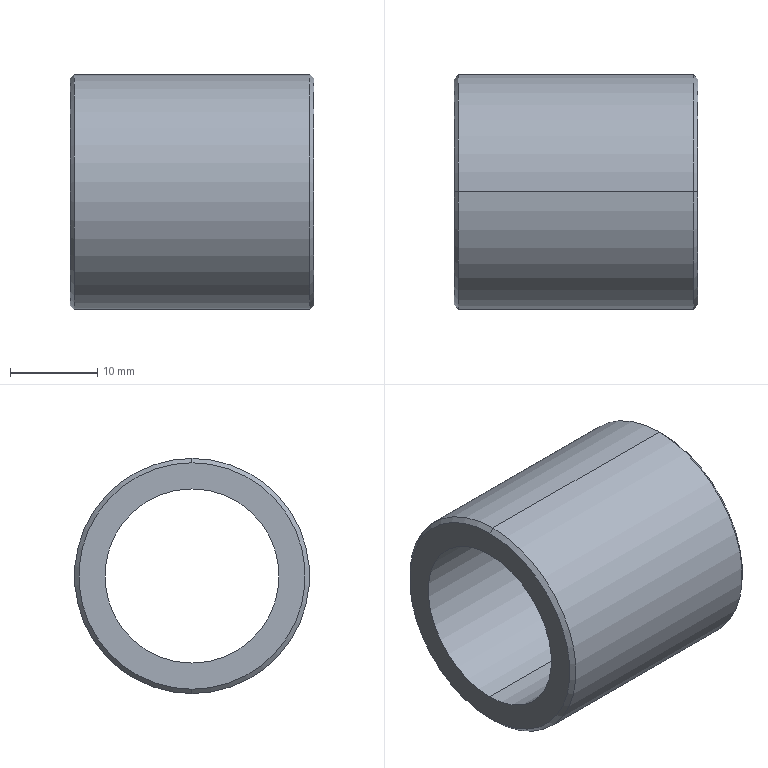Part | STEP file | CLBUS20-27-28.0-1 | 1 solid | 10 faces | box 28 x 27 x 27 mm | volume 7214 mm3 | cone 4 | cylinder 4 | plane 2 | commonest cylinder face diameters 20 x2 27 x2
STEP:
#1=CARTESIAN_POINT('',(28.,0.,-13.));
#2=VERTEX_POINT('',#1);
#3=CARTESIAN_POINT('',(28.,0.,13.));
#4=VERTEX_POINT('',#3);
#5=CARTESIAN_POINT('',(28.,0.,0.));
#6=DIRECTION('',(1.,0.,0.));
#7=DIRECTION('',(0.,0.,1.));
#8=AXIS2_PLACEMENT_3D('',#5,#6,#7);
#9=CIRCLE('',#8,13.);
#10=EDGE_CURVE('',#2,#4,#9,.T.);
#11=ORIENTED_EDGE('',*,*,#10,.F.);
#12=CARTESIAN_POINT('',(27.5,0.,-13.5));
#13=VERTEX_POINT('',#12);
#14=CARTESIAN_POINT('',(27.5,0.,-13.5));
#15=DIRECTION('',(-0.7071,0.,-0.7071));
#16=VECTOR('',#15,1000.);
#17=LINE('',#14,#16);
#18=EDGE_CURVE('',#2,#13,#17,.T.);
#19=ORIENTED_EDGE('',*,*,#18,.T.);
#20=CARTESIAN_POINT('',(27.5,0.,13.5));
#21=VERTEX_POINT('',#20);
#22=CARTESIAN_POINT('',(27.5,0.,0.));
#23=DIRECTION('',(-1.,0.,0.));
#24=DIRECTION('',(0.,0.,1.));
#25=AXIS2_PLACEMENT_3D('',#22,#23,#24);
#26=CIRCLE('',#25,13.5);
#27=EDGE_CURVE('',#21,#13,#26,.T.);
#28=ORIENTED_EDGE('',*,*,#27,.F.);
#29=CARTESIAN_POINT('',(27.5,0.,13.5));
#30=DIRECTION('',(-0.7071,0.,0.7071));
#31=VECTOR('',#30,1000.);
#32=LINE('',#29,#31);
#33=EDGE_CURVE('',#4,#21,#32,.T.);
#34=ORIENTED_EDGE('',*,*,#33,.F.);
#35=EDGE_LOOP('',(#11,#19,#28,#34));
#36=FACE_OUTER_BOUND('',#35,.T.);
#37=CARTESIAN_POINT('',(27.5,0.,0.));
#38=DIRECTION('',(-1.,0.,0.));
#39=DIRECTION('',(0.,0.,1.));
#40=AXIS2_PLACEMENT_3D('',#37,#38,#39);
#41=CONICAL_SURFACE('',#40,13.5,0.7854);
#42=ADVANCED_FACE('',(#36),#41,.T.);
#43=CARTESIAN_POINT('',(0.,0.,13.));
#44=VERTEX_POINT('',#43);
#45=CARTESIAN_POINT('',(0.,0.,-13.));
#46=VERTEX_POINT('',#45);
#47=CARTESIAN_POINT('',(0.,0.,0.));
#48=DIRECTION('',(-1.,0.,0.));
#49=DIRECTION('',(0.,0.,-1.));
#50=AXIS2_PLACEMENT_3D('',#47,#48,#49);
#51=CIRCLE('',#50,13.);
#52=EDGE_CURVE('',#44,#46,#51,.T.);
#53=ORIENTED_EDGE('',*,*,#52,.F.);
#54=CARTESIAN_POINT('',(0.5,0.,13.5));
#55=VERTEX_POINT('',#54);
#56=CARTESIAN_POINT('',(0.,0.,13.));
#57=DIRECTION('',(0.7071,0.,0.7071));
#58=VECTOR('',#57,1000.);
#59=LINE('',#56,#58);
#60=EDGE_CURVE('',#44,#55,#59,.T.);
#61=ORIENTED_EDGE('',*,*,#60,.T.);
#62=CARTESIAN_POINT('',(0.5,0.,-13.5));
#63=VERTEX_POINT('',#62);
#64=CARTESIAN_POINT('',(0.5,0.,0.));
#65=DIRECTION('',(1.,0.,0.));
#66=DIRECTION('',(0.,0.,-1.));
#67=AXIS2_PLACEMENT_3D('',#64,#65,#66);
#68=CIRCLE('',#67,13.5);
#69=EDGE_CURVE('',#63,#55,#68,.T.);
#70=ORIENTED_EDGE('',*,*,#69,.F.);
#71=CARTESIAN_POINT('',(0.,0.,-13.));
#72=DIRECTION('',(0.7071,0.,-0.7071));
#73=VECTOR('',#72,1000.);
#74=LINE('',#71,#73);
#75=EDGE_CURVE('',#46,#63,#74,.T.);
#76=ORIENTED_EDGE('',*,*,#75,.F.);
#77=EDGE_LOOP('',(#53,#61,#70,#76));
#78=FACE_OUTER_BOUND('',#77,.T.);
#79=CARTESIAN_POINT('',(0.,0.,0.));
#80=DIRECTION('',(1.,0.,0.));
#81=DIRECTION('',(0.,0.,-1.));
#82=AXIS2_PLACEMENT_3D('',#79,#80,#81);
#83=CONICAL_SURFACE('',#82,13.,0.7854);
#84=ADVANCED_FACE('',(#78),#83,.T.);
#85=ORIENTED_EDGE('',*,*,#27,.T.);
#86=CARTESIAN_POINT('',(0.,0.,-13.5));
#87=DIRECTION('',(-1.,0.,0.));
#88=VECTOR('',#87,1000.);
#89=LINE('',#86,#88);
#90=EDGE_CURVE('',#13,#63,#89,.T.);
#91=ORIENTED_EDGE('',*,*,#90,.T.);
#92=ORIENTED_EDGE('',*,*,#69,.T.);
#93=CARTESIAN_POINT('',(0.,0.,13.5));
#94=DIRECTION('',(-1.,0.,0.));
#95=VECTOR('',#94,1000.);
#96=LINE('',#93,#95);
#97=EDGE_CURVE('',#21,#55,#96,.T.);
#98=ORIENTED_EDGE('',*,*,#97,.F.);
#99=EDGE_LOOP('',(#85,#91,#92,#98));
#100=FACE_OUTER_BOUND('',#99,.T.);
#101=CARTESIAN_POINT('',(0.,0.,0.));
#102=DIRECTION('',(-1.,0.,0.));
#103=DIRECTION('',(0.,0.,1.));
#104=AXIS2_PLACEMENT_3D('',#101,#102,#103);
#105=CYLINDRICAL_SURFACE('',#104,13.5);
#106=ADVANCED_FACE('',(#100),#105,.T.);
#107=CARTESIAN_POINT('',(28.,0.,-10.));
#108=VERTEX_POINT('',#107);
#109=CARTESIAN_POINT('',(28.,0.,10.));
#110=VERTEX_POINT('',#109);
#111=CARTESIAN_POINT('',(28.,0.,0.));
#112=DIRECTION('',(-1.,0.,0.));
#113=DIRECTION('',(0.,0.,1.));
#114=AXIS2_PLACEMENT_3D('',#111,#112,#113);
#115=CIRCLE('',#114,10.);
#116=EDGE_CURVE('',#108,#110,#115,.T.);
#117=ORIENTED_EDGE('',*,*,#116,.F.);
#118=CARTESIAN_POINT('',(0.,0.,-10.));
#119=VERTEX_POINT('',#118);
#120=CARTESIAN_POINT('',(0.,0.,-10.));
#121=DIRECTION('',(-1.,0.,0.));
#122=VECTOR('',#121,1000.);
#123=LINE('',#120,#122);
#124=EDGE_CURVE('',#108,#119,#123,.T.);
#125=ORIENTED_EDGE('',*,*,#124,.T.);
#126=CARTESIAN_POINT('',(0.,0.,10.));
#127=VERTEX_POINT('',#126);
#128=CARTESIAN_POINT('',(0.,0.,0.));
#129=DIRECTION('',(-1.,0.,0.));
#130=DIRECTION('',(0.,0.,1.));
#131=AXIS2_PLACEMENT_3D('',#128,#129,#130);
#132=CIRCLE('',#131,10.);
#133=EDGE_CURVE('',#119,#127,#132,.T.);
#134=ORIENTED_EDGE('',*,*,#133,.T.);
#135=CARTESIAN_POINT('',(0.,0.,10.));
#136=DIRECTION('',(-1.,0.,0.));
#137=VECTOR('',#136,1000.);
#138=LINE('',#135,#137);
#139=EDGE_CURVE('',#110,#127,#138,.T.);
#140=ORIENTED_EDGE('',*,*,#139,.F.);
#141=EDGE_LOOP('',(#117,#125,#134,#140));
#142=FACE_OUTER_BOUND('',#141,.T.);
#143=CARTESIAN_POINT('',(0.,0.,0.));
#144=DIRECTION('',(-1.,0.,0.));
#145=DIRECTION('',(0.,0.,1.));
#146=AXIS2_PLACEMENT_3D('',#143,#144,#145);
#147=CYLINDRICAL_SURFACE('',#146,10.);
#148=ADVANCED_FACE('',(#142),#147,.F.);
#149=CARTESIAN_POINT('',(28.,0.,0.));
#150=DIRECTION('',(1.,0.,0.));
#151=DIRECTION('',(0.,0.,1.));
#152=AXIS2_PLACEMENT_3D('',#149,#150,#151);
#153=CIRCLE('',#152,13.);
#154=EDGE_CURVE('',#4,#2,#153,.T.);
#155=ORIENTED_EDGE('',*,*,#154,.T.);
#156=ORIENTED_EDGE('',*,*,#10,.T.);
#157=EDGE_LOOP('',(#155,#156));
#158=FACE_OUTER_BOUND('',#157,.T.);
#159=CARTESIAN_POINT('',(28.,0.,0.));
#160=DIRECTION('',(-1.,0.,0.));
#161=DIRECTION('',(0.,0.,1.));
#162=AXIS2_PLACEMENT_3D('',#159,#160,#161);
#163=CIRCLE('',#162,10.);
#164=EDGE_CURVE('',#110,#108,#163,.T.);
#165=ORIENTED_EDGE('',*,*,#164,.T.);
#166=ORIENTED_EDGE('',*,*,#116,.T.);
#167=EDGE_LOOP('',(#165,#166));
#168=FACE_BOUND('',#167,.T.);
#169=CARTESIAN_POINT('',(28.,13.5,0.));
#170=DIRECTION('',(-1.,0.,0.));
#171=DIRECTION('',(0.,0.,1.));
#172=AXIS2_PLACEMENT_3D('',#169,#170,#171);
#173=PLANE('',#172);
#174=ADVANCED_FACE('',(#158,#168),#173,.F.);
#175=ORIENTED_EDGE('',*,*,#124,.F.);
#176=ORIENTED_EDGE('',*,*,#164,.F.);
#177=ORIENTED_EDGE('',*,*,#139,.T.);
#178=CARTESIAN_POINT('',(0.,0.,0.));
#179=DIRECTION('',(-1.,0.,0.));
#180=DIRECTION('',(0.,0.,1.));
#181=AXIS2_PLACEMENT_3D('',#178,#179,#180);
#182=CIRCLE('',#181,10.);
#183=EDGE_CURVE('',#127,#119,#182,.T.);
#184=ORIENTED_EDGE('',*,*,#183,.T.);
#185=EDGE_LOOP('',(#175,#176,#177,#184));
#186=FACE_OUTER_BOUND('',#185,.T.);
#187=CARTESIAN_POINT('',(0.,0.,0.));
#188=DIRECTION('',(-1.,0.,0.));
#189=DIRECTION('',(0.,0.,1.));
#190=AXIS2_PLACEMENT_3D('',#187,#188,#189);
#191=CYLINDRICAL_SURFACE('',#190,10.);
#192=ADVANCED_FACE('',(#186),#191,.F.);
#193=CARTESIAN_POINT('',(0.,0.,0.));
#194=DIRECTION('',(-1.,0.,0.));
#195=DIRECTION('',(0.,0.,-1.));
#196=AXIS2_PLACEMENT_3D('',#193,#194,#195);
#197=CIRCLE('',#196,13.);
#198=EDGE_CURVE('',#46,#44,#197,.T.);
#199=ORIENTED_EDGE('',*,*,#198,.T.);
#200=ORIENTED_EDGE('',*,*,#52,.T.);
#201=EDGE_LOOP('',(#199,#200));
#202=FACE_OUTER_BOUND('',#201,.T.);
#203=ORIENTED_EDGE('',*,*,#183,.F.);
#204=ORIENTED_EDGE('',*,*,#133,.F.);
#205=EDGE_LOOP('',(#203,#204));
#206=FACE_BOUND('',#205,.T.);
#207=CARTESIAN_POINT('',(0.,10.,0.));
#208=DIRECTION('',(1.,0.,0.));
#209=DIRECTION('',(0.,0.,-1.));
#210=AXIS2_PLACEMENT_3D('',#207,#208,#209);
#211=PLANE('',#210);
#212=ADVANCED_FACE('',(#202,#206),#211,.F.);
#213=ORIENTED_EDGE('',*,*,#90,.F.);
#214=CARTESIAN_POINT('',(27.5,0.,0.));
#215=DIRECTION('',(-1.,0.,0.));
#216=DIRECTION('',(0.,0.,1.));
#217=AXIS2_PLACEMENT_3D('',#214,#215,#216);
#218=CIRCLE('',#217,13.5);
#219=EDGE_CURVE('',#13,#21,#218,.T.);
#220=ORIENTED_EDGE('',*,*,#219,.T.);
#221=ORIENTED_EDGE('',*,*,#97,.T.);
#222=CARTESIAN_POINT('',(0.5,0.,0.));
#223=DIRECTION('',(1.,0.,0.));
#224=DIRECTION('',(0.,0.,-1.));
#225=AXIS2_PLACEMENT_3D('',#222,#223,#224);
#226=CIRCLE('',#225,13.5);
#227=EDGE_CURVE('',#55,#63,#226,.T.);
#228=ORIENTED_EDGE('',*,*,#227,.T.);
#229=EDGE_LOOP('',(#213,#220,#221,#228));
#230=FACE_OUTER_BOUND('',#229,.T.);
#231=CARTESIAN_POINT('',(0.,0.,0.));
#232=DIRECTION('',(-1.,0.,0.));
#233=DIRECTION('',(0.,0.,1.));
#234=AXIS2_PLACEMENT_3D('',#231,#232,#233);
#235=CYLINDRICAL_SURFACE('',#234,13.5);
#236=ADVANCED_FACE('',(#230),#235,.T.);
#237=ORIENTED_EDGE('',*,*,#60,.F.);
#238=ORIENTED_EDGE('',*,*,#198,.F.);
#239=ORIENTED_EDGE('',*,*,#75,.T.);
#240=ORIENTED_EDGE('',*,*,#227,.F.);
#241=EDGE_LOOP('',(#237,#238,#239,#240));
#242=FACE_OUTER_BOUND('',#241,.T.);
#243=CARTESIAN_POINT('',(0.,0.,0.));
#244=DIRECTION('',(1.,0.,0.));
#245=DIRECTION('',(0.,0.,-1.));
#246=AXIS2_PLACEMENT_3D('',#243,#244,#245);
#247=CONICAL_SURFACE('',#246,13.,0.7854);
#248=ADVANCED_FACE('',(#242),#247,.T.);
#249=ORIENTED_EDGE('',*,*,#18,.F.);
#250=ORIENTED_EDGE('',*,*,#154,.F.);
#251=ORIENTED_EDGE('',*,*,#33,.T.);
#252=ORIENTED_EDGE('',*,*,#219,.F.);
#253=EDGE_LOOP('',(#249,#250,#251,#252));
#254=FACE_OUTER_BOUND('',#253,.T.);
#255=CARTESIAN_POINT('',(27.5,0.,0.));
#256=DIRECTION('',(-1.,0.,0.));
#257=DIRECTION('',(0.,0.,1.));
#258=AXIS2_PLACEMENT_3D('',#255,#256,#257);
#259=CONICAL_SURFACE('',#258,13.5,0.7854);
#260=ADVANCED_FACE('',(#254),#259,.T.);
#261=CLOSED_SHELL('',(#42,#84,#106,#148,#174,#192,#212,#236,#248,#260));
#262=MANIFOLD_SOLID_BREP('',#261);
#263=CARTESIAN_POINT('',(0.,0.,0.));
#264=DIRECTION('',(0.,0.,1.));
#265=DIRECTION('',(1.,0.,0.));
#266=AXIS2_PLACEMENT_3D('',#263,#264,#265);
#267=(LENGTH_UNIT()NAMED_UNIT(*)SI_UNIT(.MILLI.,.METRE.));
#268=UNCERTAINTY_MEASURE_WITH_UNIT(LENGTH_MEASURE(0.00001),#267,'','');
#269=(NAMED_UNIT(*)PLANE_ANGLE_UNIT()SI_UNIT($,.RADIAN.));
#270=(NAMED_UNIT(*)SI_UNIT($,.STERADIAN.)SOLID_ANGLE_UNIT());
#271=(GEOMETRIC_REPRESENTATION_CONTEXT(3)GLOBAL_UNCERTAINTY_ASSIGNED_CONTEXT((#268))GLOBAL_UNIT_ASSIGNED_CONTEXT((#267,#269,#270))REPRESENTATION_CONTEXT('',''));
#272=ADVANCED_BREP_SHAPE_REPRESENTATION('',(#262,#266),#271);